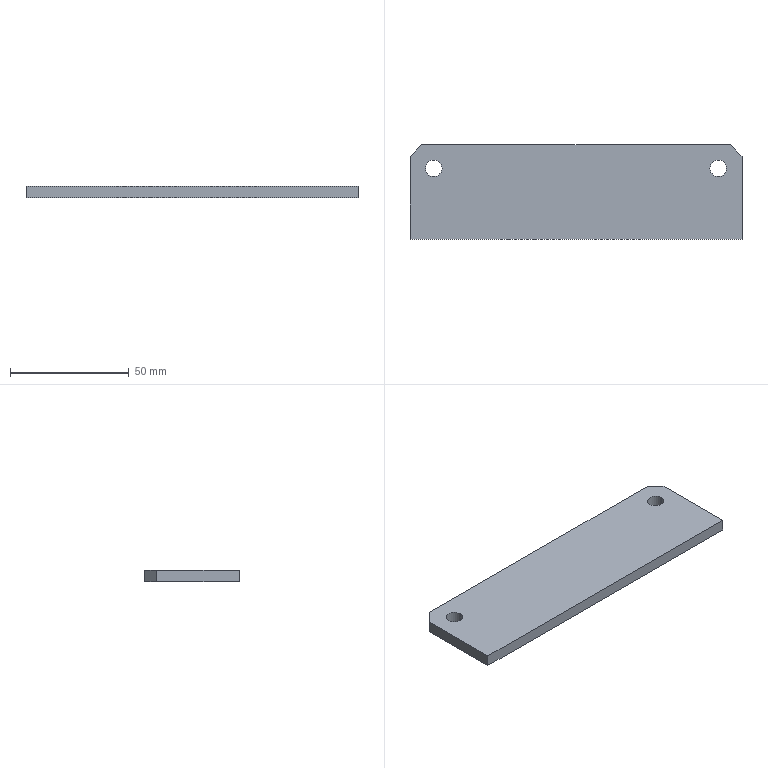Part | SolidWorks | features Chamfer 1, Extrusion 1, ICE 1 | 1 solid | 12 faces | box 140 x 40 x 5 mm | volume 27490 mm3 | plane 8 | cylinder 4 | commonest cylinder face diameters 7 x4
STEP:
#1=CARTESIAN_POINT('',(-63.5,10.,0.));
#2=VERTEX_POINT('',#1);
#3=CARTESIAN_POINT('',(-56.5,10.,0.));
#4=VERTEX_POINT('',#3);
#5=CARTESIAN_POINT('',(-60.,10.,0.));
#6=DIRECTION('',(0.,0.,1.));
#7=DIRECTION('',(1.,0.,0.));
#8=AXIS2_PLACEMENT_3D('',#5,#6,#7);
#9=CIRCLE('',#8,3.5);
#10=EDGE_CURVE('',#2,#4,#9,.T.);
#11=ORIENTED_EDGE('',*,*,#10,.F.);
#12=CARTESIAN_POINT('',(-63.5,10.,5.));
#13=VERTEX_POINT('',#12);
#14=CARTESIAN_POINT('',(-63.5,10.,0.));
#15=DIRECTION('',(0.,0.,1.));
#16=VECTOR('',#15,1000.);
#17=LINE('',#14,#16);
#18=EDGE_CURVE('',#2,#13,#17,.T.);
#19=ORIENTED_EDGE('',*,*,#18,.T.);
#20=CARTESIAN_POINT('',(-56.5,10.,5.));
#21=VERTEX_POINT('',#20);
#22=CARTESIAN_POINT('',(-60.,10.,5.));
#23=DIRECTION('',(0.,0.,1.));
#24=DIRECTION('',(1.,0.,0.));
#25=AXIS2_PLACEMENT_3D('',#22,#23,#24);
#26=CIRCLE('',#25,3.5);
#27=EDGE_CURVE('',#13,#21,#26,.T.);
#28=ORIENTED_EDGE('',*,*,#27,.T.);
#29=CARTESIAN_POINT('',(-56.5,10.,0.));
#30=DIRECTION('',(0.,0.,1.));
#31=VECTOR('',#30,1000.);
#32=LINE('',#29,#31);
#33=EDGE_CURVE('',#4,#21,#32,.T.);
#34=ORIENTED_EDGE('',*,*,#33,.F.);
#35=EDGE_LOOP('',(#11,#19,#28,#34));
#36=FACE_OUTER_BOUND('',#35,.T.);
#37=CARTESIAN_POINT('',(-60.,10.,0.));
#38=DIRECTION('',(0.,0.,1.));
#39=DIRECTION('',(1.,0.,0.));
#40=AXIS2_PLACEMENT_3D('',#37,#38,#39);
#41=CYLINDRICAL_SURFACE('',#40,3.5);
#42=ADVANCED_FACE('',(#36),#41,.F.);
#43=CARTESIAN_POINT('',(56.5,10.,0.));
#44=VERTEX_POINT('',#43);
#45=CARTESIAN_POINT('',(63.5,10.,0.));
#46=VERTEX_POINT('',#45);
#47=CARTESIAN_POINT('',(60.,10.,0.));
#48=DIRECTION('',(0.,0.,1.));
#49=DIRECTION('',(1.,0.,0.));
#50=AXIS2_PLACEMENT_3D('',#47,#48,#49);
#51=CIRCLE('',#50,3.5);
#52=EDGE_CURVE('',#44,#46,#51,.T.);
#53=ORIENTED_EDGE('',*,*,#52,.F.);
#54=CARTESIAN_POINT('',(56.5,10.,5.));
#55=VERTEX_POINT('',#54);
#56=CARTESIAN_POINT('',(56.5,10.,0.));
#57=DIRECTION('',(0.,0.,1.));
#58=VECTOR('',#57,1000.);
#59=LINE('',#56,#58);
#60=EDGE_CURVE('',#44,#55,#59,.T.);
#61=ORIENTED_EDGE('',*,*,#60,.T.);
#62=CARTESIAN_POINT('',(63.5,10.,5.));
#63=VERTEX_POINT('',#62);
#64=CARTESIAN_POINT('',(60.,10.,5.));
#65=DIRECTION('',(0.,0.,1.));
#66=DIRECTION('',(1.,0.,0.));
#67=AXIS2_PLACEMENT_3D('',#64,#65,#66);
#68=CIRCLE('',#67,3.5);
#69=EDGE_CURVE('',#55,#63,#68,.T.);
#70=ORIENTED_EDGE('',*,*,#69,.T.);
#71=CARTESIAN_POINT('',(63.5,10.,0.));
#72=DIRECTION('',(0.,0.,1.));
#73=VECTOR('',#72,1000.);
#74=LINE('',#71,#73);
#75=EDGE_CURVE('',#46,#63,#74,.T.);
#76=ORIENTED_EDGE('',*,*,#75,.F.);
#77=EDGE_LOOP('',(#53,#61,#70,#76));
#78=FACE_OUTER_BOUND('',#77,.T.);
#79=CARTESIAN_POINT('',(60.,10.,0.));
#80=DIRECTION('',(0.,0.,1.));
#81=DIRECTION('',(1.,0.,0.));
#82=AXIS2_PLACEMENT_3D('',#79,#80,#81);
#83=CYLINDRICAL_SURFACE('',#82,3.5);
#84=ADVANCED_FACE('',(#78),#83,.F.);
#85=CARTESIAN_POINT('',(-70.,15.,5.));
#86=VERTEX_POINT('',#85);
#87=CARTESIAN_POINT('',(-70.,-20.,5.));
#88=VERTEX_POINT('',#87);
#89=CARTESIAN_POINT('',(-70.,20.,5.));
#90=DIRECTION('',(0.,-1.,0.));
#91=VECTOR('',#90,1000.);
#92=LINE('',#89,#91);
#93=EDGE_CURVE('',#86,#88,#92,.T.);
#94=ORIENTED_EDGE('',*,*,#93,.F.);
#95=CARTESIAN_POINT('',(-70.,15.,0.));
#96=VERTEX_POINT('',#95);
#97=CARTESIAN_POINT('',(-70.,15.,5.));
#98=DIRECTION('',(0.,0.,-1.));
#99=VECTOR('',#98,1000.);
#100=LINE('',#97,#99);
#101=EDGE_CURVE('',#86,#96,#100,.T.);
#102=ORIENTED_EDGE('',*,*,#101,.T.);
#103=CARTESIAN_POINT('',(-70.,-20.,0.));
#104=VERTEX_POINT('',#103);
#105=CARTESIAN_POINT('',(-70.,20.,0.));
#106=DIRECTION('',(0.,-1.,0.));
#107=VECTOR('',#106,1000.);
#108=LINE('',#105,#107);
#109=EDGE_CURVE('',#96,#104,#108,.T.);
#110=ORIENTED_EDGE('',*,*,#109,.T.);
#111=CARTESIAN_POINT('',(-70.,-20.,5.));
#112=DIRECTION('',(0.,0.,-1.));
#113=VECTOR('',#112,1000.);
#114=LINE('',#111,#113);
#115=EDGE_CURVE('',#88,#104,#114,.T.);
#116=ORIENTED_EDGE('',*,*,#115,.F.);
#117=EDGE_LOOP('',(#94,#102,#110,#116));
#118=FACE_OUTER_BOUND('',#117,.T.);
#119=CARTESIAN_POINT('',(-70.,20.,5.));
#120=DIRECTION('',(1.,0.,0.));
#121=DIRECTION('',(0.,1.,0.));
#122=AXIS2_PLACEMENT_3D('',#119,#120,#121);
#123=PLANE('',#122);
#124=ADVANCED_FACE('',(#118),#123,.F.);
#125=CARTESIAN_POINT('',(70.,-20.,0.));
#126=VERTEX_POINT('',#125);
#127=CARTESIAN_POINT('',(70.,-20.,0.));
#128=DIRECTION('',(1.,0.,0.));
#129=VECTOR('',#128,1000.);
#130=LINE('',#127,#129);
#131=EDGE_CURVE('',#104,#126,#130,.T.);
#132=ORIENTED_EDGE('',*,*,#131,.T.);
#133=CARTESIAN_POINT('',(70.,-20.,5.));
#134=VERTEX_POINT('',#133);
#135=CARTESIAN_POINT('',(70.,-20.,5.));
#136=DIRECTION('',(0.,0.,-1.));
#137=VECTOR('',#136,1000.);
#138=LINE('',#135,#137);
#139=EDGE_CURVE('',#134,#126,#138,.T.);
#140=ORIENTED_EDGE('',*,*,#139,.F.);
#141=CARTESIAN_POINT('',(70.,-20.,5.));
#142=DIRECTION('',(1.,0.,0.));
#143=VECTOR('',#142,1000.);
#144=LINE('',#141,#143);
#145=EDGE_CURVE('',#88,#134,#144,.T.);
#146=ORIENTED_EDGE('',*,*,#145,.F.);
#147=ORIENTED_EDGE('',*,*,#115,.T.);
#148=EDGE_LOOP('',(#132,#140,#146,#147));
#149=FACE_OUTER_BOUND('',#148,.T.);
#150=CARTESIAN_POINT('',(70.,-20.,5.));
#151=DIRECTION('',(0.,1.,0.));
#152=DIRECTION('',(-1.,0.,0.));
#153=AXIS2_PLACEMENT_3D('',#150,#151,#152);
#154=PLANE('',#153);
#155=ADVANCED_FACE('',(#149),#154,.F.);
#156=CARTESIAN_POINT('',(70.,15.,0.));
#157=VERTEX_POINT('',#156);
#158=CARTESIAN_POINT('',(70.,20.,0.));
#159=DIRECTION('',(0.,1.,0.));
#160=VECTOR('',#159,1000.);
#161=LINE('',#158,#160);
#162=EDGE_CURVE('',#126,#157,#161,.T.);
#163=ORIENTED_EDGE('',*,*,#162,.T.);
#164=CARTESIAN_POINT('',(70.,15.,5.));
#165=VERTEX_POINT('',#164);
#166=CARTESIAN_POINT('',(70.,15.,5.));
#167=DIRECTION('',(0.,0.,1.));
#168=VECTOR('',#167,1000.);
#169=LINE('',#166,#168);
#170=EDGE_CURVE('',#157,#165,#169,.T.);
#171=ORIENTED_EDGE('',*,*,#170,.T.);
#172=CARTESIAN_POINT('',(70.,20.,5.));
#173=DIRECTION('',(0.,1.,0.));
#174=VECTOR('',#173,1000.);
#175=LINE('',#172,#174);
#176=EDGE_CURVE('',#134,#165,#175,.T.);
#177=ORIENTED_EDGE('',*,*,#176,.F.);
#178=ORIENTED_EDGE('',*,*,#139,.T.);
#179=EDGE_LOOP('',(#163,#171,#177,#178));
#180=FACE_OUTER_BOUND('',#179,.T.);
#181=CARTESIAN_POINT('',(70.,20.,5.));
#182=DIRECTION('',(-1.,0.,0.));
#183=DIRECTION('',(0.,0.,1.));
#184=AXIS2_PLACEMENT_3D('',#181,#182,#183);
#185=PLANE('',#184);
#186=ADVANCED_FACE('',(#180),#185,.F.);
#187=CARTESIAN_POINT('',(65.,20.,5.));
#188=VERTEX_POINT('',#187);
#189=CARTESIAN_POINT('',(-65.,20.,5.));
#190=VERTEX_POINT('',#189);
#191=CARTESIAN_POINT('',(70.,20.,5.));
#192=DIRECTION('',(-1.,0.,0.));
#193=VECTOR('',#192,1000.);
#194=LINE('',#191,#193);
#195=EDGE_CURVE('',#188,#190,#194,.T.);
#196=ORIENTED_EDGE('',*,*,#195,.F.);
#197=CARTESIAN_POINT('',(65.,20.,0.));
#198=VERTEX_POINT('',#197);
#199=CARTESIAN_POINT('',(65.,20.,5.));
#200=DIRECTION('',(0.,0.,-1.));
#201=VECTOR('',#200,1000.);
#202=LINE('',#199,#201);
#203=EDGE_CURVE('',#188,#198,#202,.T.);
#204=ORIENTED_EDGE('',*,*,#203,.T.);
#205=CARTESIAN_POINT('',(-65.,20.,0.));
#206=VERTEX_POINT('',#205);
#207=CARTESIAN_POINT('',(70.,20.,0.));
#208=DIRECTION('',(-1.,0.,0.));
#209=VECTOR('',#208,1000.);
#210=LINE('',#207,#209);
#211=EDGE_CURVE('',#198,#206,#210,.T.);
#212=ORIENTED_EDGE('',*,*,#211,.T.);
#213=CARTESIAN_POINT('',(-65.,20.,5.));
#214=DIRECTION('',(0.,0.,1.));
#215=VECTOR('',#214,1000.);
#216=LINE('',#213,#215);
#217=EDGE_CURVE('',#206,#190,#216,.T.);
#218=ORIENTED_EDGE('',*,*,#217,.T.);
#219=EDGE_LOOP('',(#196,#204,#212,#218));
#220=FACE_OUTER_BOUND('',#219,.T.);
#221=CARTESIAN_POINT('',(70.,20.,5.));
#222=DIRECTION('',(0.,-1.,0.));
#223=DIRECTION('',(1.,0.,0.));
#224=AXIS2_PLACEMENT_3D('',#221,#222,#223);
#225=PLANE('',#224);
#226=ADVANCED_FACE('',(#220),#225,.F.);
#227=CARTESIAN_POINT('',(-60.,10.,5.));
#228=DIRECTION('',(0.,0.,1.));
#229=DIRECTION('',(1.,0.,0.));
#230=AXIS2_PLACEMENT_3D('',#227,#228,#229);
#231=CIRCLE('',#230,3.5);
#232=EDGE_CURVE('',#21,#13,#231,.T.);
#233=ORIENTED_EDGE('',*,*,#232,.F.);
#234=ORIENTED_EDGE('',*,*,#27,.F.);
#235=EDGE_LOOP('',(#233,#234));
#236=FACE_BOUND('',#235,.T.);
#237=CARTESIAN_POINT('',(60.,10.,5.));
#238=DIRECTION('',(0.,0.,1.));
#239=DIRECTION('',(1.,0.,0.));
#240=AXIS2_PLACEMENT_3D('',#237,#238,#239);
#241=CIRCLE('',#240,3.5);
#242=EDGE_CURVE('',#63,#55,#241,.T.);
#243=ORIENTED_EDGE('',*,*,#242,.F.);
#244=ORIENTED_EDGE('',*,*,#69,.F.);
#245=EDGE_LOOP('',(#243,#244));
#246=FACE_BOUND('',#245,.T.);
#247=ORIENTED_EDGE('',*,*,#176,.T.);
#248=CARTESIAN_POINT('',(65.,20.,5.));
#249=DIRECTION('',(-0.7071,0.7071,0.));
#250=VECTOR('',#249,1000.);
#251=LINE('',#248,#250);
#252=EDGE_CURVE('',#165,#188,#251,.T.);
#253=ORIENTED_EDGE('',*,*,#252,.T.);
#254=ORIENTED_EDGE('',*,*,#195,.T.);
#255=CARTESIAN_POINT('',(-70.,15.,5.));
#256=DIRECTION('',(-0.7071,-0.7071,0.));
#257=VECTOR('',#256,1000.);
#258=LINE('',#255,#257);
#259=EDGE_CURVE('',#190,#86,#258,.T.);
#260=ORIENTED_EDGE('',*,*,#259,.T.);
#261=ORIENTED_EDGE('',*,*,#93,.T.);
#262=ORIENTED_EDGE('',*,*,#145,.T.);
#263=EDGE_LOOP('',(#247,#253,#254,#260,#261,#262));
#264=FACE_OUTER_BOUND('',#263,.T.);
#265=CARTESIAN_POINT('',(0.,0.,5.));
#266=DIRECTION('',(0.,0.,-1.));
#267=DIRECTION('',(-1.,0.,0.));
#268=AXIS2_PLACEMENT_3D('',#265,#266,#267);
#269=PLANE('',#268);
#270=ADVANCED_FACE('',(#236,#246,#264),#269,.F.);
#271=CARTESIAN_POINT('',(-60.,10.,0.));
#272=DIRECTION('',(0.,0.,1.));
#273=DIRECTION('',(1.,0.,0.));
#274=AXIS2_PLACEMENT_3D('',#271,#272,#273);
#275=CIRCLE('',#274,3.5);
#276=EDGE_CURVE('',#4,#2,#275,.T.);
#277=ORIENTED_EDGE('',*,*,#276,.T.);
#278=ORIENTED_EDGE('',*,*,#10,.T.);
#279=EDGE_LOOP('',(#277,#278));
#280=FACE_BOUND('',#279,.T.);
#281=CARTESIAN_POINT('',(60.,10.,0.));
#282=DIRECTION('',(0.,0.,1.));
#283=DIRECTION('',(1.,0.,0.));
#284=AXIS2_PLACEMENT_3D('',#281,#282,#283);
#285=CIRCLE('',#284,3.5);
#286=EDGE_CURVE('',#46,#44,#285,.T.);
#287=ORIENTED_EDGE('',*,*,#286,.T.);
#288=ORIENTED_EDGE('',*,*,#52,.T.);
#289=EDGE_LOOP('',(#287,#288));
#290=FACE_BOUND('',#289,.T.);
#291=ORIENTED_EDGE('',*,*,#211,.F.);
#292=CARTESIAN_POINT('',(42.5,42.5,0.));
#293=DIRECTION('',(0.7071,-0.7071,0.));
#294=VECTOR('',#293,1000.);
#295=LINE('',#292,#294);
#296=EDGE_CURVE('',#198,#157,#295,.T.);
#297=ORIENTED_EDGE('',*,*,#296,.T.);
#298=ORIENTED_EDGE('',*,*,#162,.F.);
#299=ORIENTED_EDGE('',*,*,#131,.F.);
#300=ORIENTED_EDGE('',*,*,#109,.F.);
#301=CARTESIAN_POINT('',(-42.5,42.5,0.));
#302=DIRECTION('',(0.7071,0.7071,0.));
#303=VECTOR('',#302,1000.);
#304=LINE('',#301,#303);
#305=EDGE_CURVE('',#96,#206,#304,.T.);
#306=ORIENTED_EDGE('',*,*,#305,.T.);
#307=EDGE_LOOP('',(#291,#297,#298,#299,#300,#306));
#308=FACE_OUTER_BOUND('',#307,.T.);
#309=CARTESIAN_POINT('',(0.,0.,0.));
#310=DIRECTION('',(0.,0.,-1.));
#311=DIRECTION('',(-1.,0.,0.));
#312=AXIS2_PLACEMENT_3D('',#309,#310,#311);
#313=PLANE('',#312);
#314=ADVANCED_FACE('',(#280,#290,#308),#313,.T.);
#315=ORIENTED_EDGE('',*,*,#60,.F.);
#316=ORIENTED_EDGE('',*,*,#286,.F.);
#317=ORIENTED_EDGE('',*,*,#75,.T.);
#318=ORIENTED_EDGE('',*,*,#242,.T.);
#319=EDGE_LOOP('',(#315,#316,#317,#318));
#320=FACE_OUTER_BOUND('',#319,.T.);
#321=CARTESIAN_POINT('',(60.,10.,0.));
#322=DIRECTION('',(0.,0.,1.));
#323=DIRECTION('',(1.,0.,0.));
#324=AXIS2_PLACEMENT_3D('',#321,#322,#323);
#325=CYLINDRICAL_SURFACE('',#324,3.5);
#326=ADVANCED_FACE('',(#320),#325,.F.);
#327=ORIENTED_EDGE('',*,*,#18,.F.);
#328=ORIENTED_EDGE('',*,*,#276,.F.);
#329=ORIENTED_EDGE('',*,*,#33,.T.);
#330=ORIENTED_EDGE('',*,*,#232,.T.);
#331=EDGE_LOOP('',(#327,#328,#329,#330));
#332=FACE_OUTER_BOUND('',#331,.T.);
#333=CARTESIAN_POINT('',(-60.,10.,0.));
#334=DIRECTION('',(0.,0.,1.));
#335=DIRECTION('',(1.,0.,0.));
#336=AXIS2_PLACEMENT_3D('',#333,#334,#335);
#337=CYLINDRICAL_SURFACE('',#336,3.5);
#338=ADVANCED_FACE('',(#332),#337,.F.);
#339=ORIENTED_EDGE('',*,*,#252,.F.);
#340=ORIENTED_EDGE('',*,*,#170,.F.);
#341=ORIENTED_EDGE('',*,*,#296,.F.);
#342=ORIENTED_EDGE('',*,*,#203,.F.);
#343=EDGE_LOOP('',(#339,#340,#341,#342));
#344=FACE_OUTER_BOUND('',#343,.T.);
#345=CARTESIAN_POINT('',(65.,20.,5.));
#346=DIRECTION('',(-0.7071,-0.7071,0.));
#347=DIRECTION('',(0.,0.,-1.));
#348=AXIS2_PLACEMENT_3D('',#345,#346,#347);
#349=PLANE('',#348);
#350=ADVANCED_FACE('',(#344),#349,.F.);
#351=ORIENTED_EDGE('',*,*,#259,.F.);
#352=ORIENTED_EDGE('',*,*,#217,.F.);
#353=ORIENTED_EDGE('',*,*,#305,.F.);
#354=ORIENTED_EDGE('',*,*,#101,.F.);
#355=EDGE_LOOP('',(#351,#352,#353,#354));
#356=FACE_OUTER_BOUND('',#355,.T.);
#357=CARTESIAN_POINT('',(-70.,15.,5.));
#358=DIRECTION('',(0.7071,-0.7071,0.));
#359=DIRECTION('',(0.,0.,-1.));
#360=AXIS2_PLACEMENT_3D('',#357,#358,#359);
#361=PLANE('',#360);
#362=ADVANCED_FACE('',(#356),#361,.F.);
#363=CLOSED_SHELL('',(#42,#84,#124,#155,#186,#226,#270,#314,#326,#338,#350,#362));
#364=MANIFOLD_SOLID_BREP('',#363);
#365=CARTESIAN_POINT('',(0.,0.,0.));
#366=DIRECTION('',(0.,0.,1.));
#367=DIRECTION('',(1.,0.,0.));
#368=AXIS2_PLACEMENT_3D('',#365,#366,#367);
#369=(LENGTH_UNIT()NAMED_UNIT(*)SI_UNIT(.MILLI.,.METRE.));
#370=UNCERTAINTY_MEASURE_WITH_UNIT(LENGTH_MEASURE(0.00001),#369,'','');
#371=(NAMED_UNIT(*)PLANE_ANGLE_UNIT()SI_UNIT($,.RADIAN.));
#372=(NAMED_UNIT(*)SI_UNIT($,.STERADIAN.)SOLID_ANGLE_UNIT());
#373=(GEOMETRIC_REPRESENTATION_CONTEXT(3)GLOBAL_UNCERTAINTY_ASSIGNED_CONTEXT((#370))GLOBAL_UNIT_ASSIGNED_CONTEXT((#369,#371,#372))REPRESENTATION_CONTEXT('',''));
#374=ADVANCED_BREP_SHAPE_REPRESENTATION('',(#364,#368),#373);